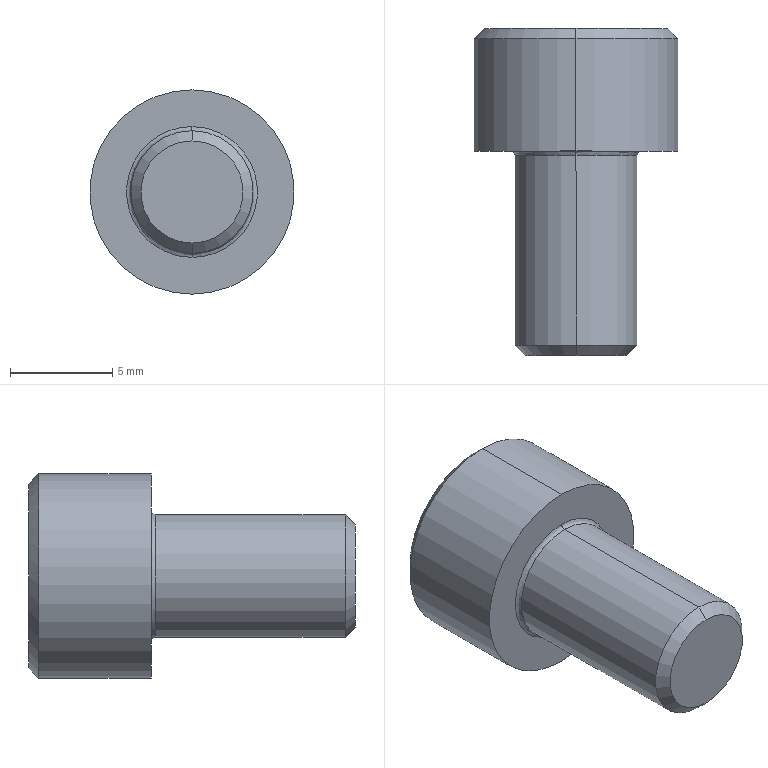Part | STEP file | 1 solid | 20 faces | box 10 x 16 x 10 mm | volume 650.705 mm3 | plane 10 | cone 4 | cylinder 4 | spline 2 | commonest cylinder face diameters 6 x2 10 x2